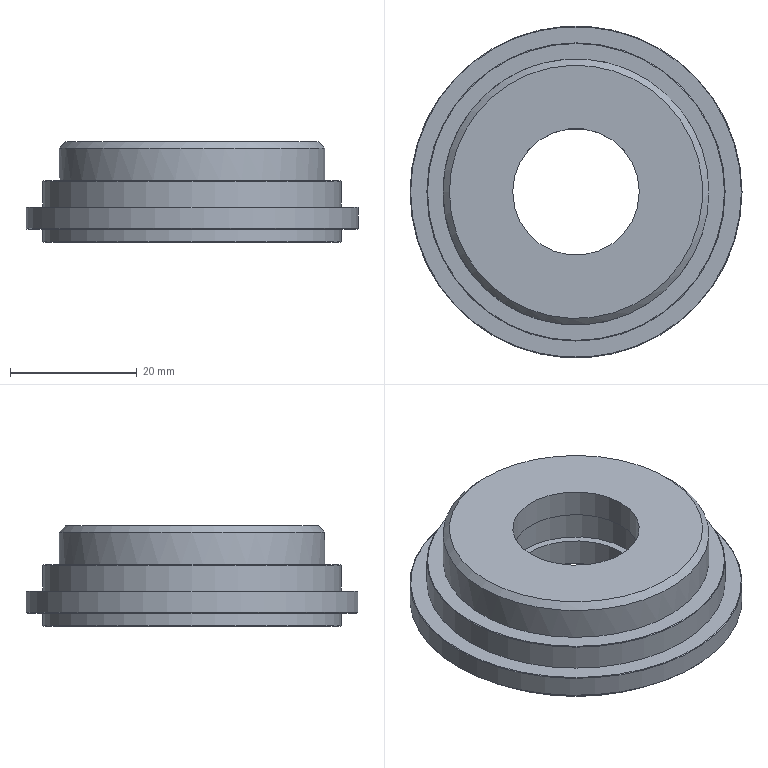Part | NX | features CHAMFER 8, DATUM_CSYS 8, SKETCH 7, EXTRUDE 6, DATUM_PLANE 5, DISTANCE MEASUREMENT 2, Resize Face 2 | 1 solid | 22 faces | box 52.42 x 52.42 x 15.88 mm | volume 19851 mm3 | cylinder 8 | plane 8 | cone 6 | commonest cylinder face diameters 20 x2 47.08 x2 22.22 x1 37.22 x1 41.98 x1 52.42 x1
STEP:
#1=CARTESIAN_POINT('',(10.,0.,11.52));
#2=VERTEX_POINT('',#1);
#3=CARTESIAN_POINT('',(0.,0.,11.52));
#4=DIRECTION('',(0.,0.,1.));
#5=DIRECTION('',(1.,0.,0.));
#6=AXIS2_PLACEMENT_3D('',#3,#4,#5);
#7=CIRCLE('',#6,10.);
#8=EDGE_CURVE('',#2,#2,#7,.T.);
#9=ORIENTED_EDGE('',*,*,#8,.F.);
#10=EDGE_LOOP('',(#9));
#11=FACE_BOUND('',#10,.T.);
#12=CARTESIAN_POINT('',(-10.,0.,15.88));
#13=VERTEX_POINT('',#12);
#14=CARTESIAN_POINT('',(0.,0.,15.88));
#15=DIRECTION('',(0.,0.,-1.));
#16=DIRECTION('',(-1.,0.,0.));
#17=AXIS2_PLACEMENT_3D('',#14,#15,#16);
#18=CIRCLE('',#17,10.);
#19=EDGE_CURVE('',#13,#13,#18,.T.);
#20=ORIENTED_EDGE('',*,*,#19,.F.);
#21=EDGE_LOOP('',(#20));
#22=FACE_BOUND('',#21,.T.);
#23=CARTESIAN_POINT('',(0.,0.,15.88));
#24=DIRECTION('',(0.,0.,-1.));
#25=DIRECTION('',(-1.,0.,0.));
#26=AXIS2_PLACEMENT_3D('',#23,#24,#25);
#27=CYLINDRICAL_SURFACE('',#26,10.);
#28=ADVANCED_FACE('',(#11,#22),#27,.F.);
#29=CARTESIAN_POINT('',(18.61,0.,2.08));
#30=VERTEX_POINT('',#29);
#31=CARTESIAN_POINT('',(0.,0.,2.08));
#32=DIRECTION('',(0.,0.,1.));
#33=DIRECTION('',(1.,0.,0.));
#34=AXIS2_PLACEMENT_3D('',#31,#32,#33);
#35=CIRCLE('',#34,18.61);
#36=EDGE_CURVE('',#30,#30,#35,.F.);
#37=ORIENTED_EDGE('',*,*,#36,.T.);
#38=EDGE_LOOP('',(#37));
#39=FACE_BOUND('',#38,.T.);
#40=CARTESIAN_POINT('',(10.,0.,2.08));
#41=VERTEX_POINT('',#40);
#42=CARTESIAN_POINT('',(0.,0.,2.08));
#43=DIRECTION('',(0.,0.,1.));
#44=DIRECTION('',(1.,0.,0.));
#45=AXIS2_PLACEMENT_3D('',#42,#43,#44);
#46=CIRCLE('',#45,10.);
#47=EDGE_CURVE('',#41,#41,#46,.F.);
#48=ORIENTED_EDGE('',*,*,#47,.F.);
#49=EDGE_LOOP('',(#48));
#50=FACE_BOUND('',#49,.T.);
#51=CARTESIAN_POINT('',(0.,0.,2.08));
#52=DIRECTION('',(0.,0.,1.));
#53=DIRECTION('',(1.,0.,0.));
#54=AXIS2_PLACEMENT_3D('',#51,#52,#53);
#55=PLANE('',#54);
#56=ADVANCED_FACE('',(#39,#50),#55,.F.);
#57=CARTESIAN_POINT('',(26.21,0.,2.18));
#58=VERTEX_POINT('',#57);
#59=CARTESIAN_POINT('',(0.,0.,2.18));
#60=DIRECTION('',(0.,0.,1.));
#61=DIRECTION('',(1.,0.,0.));
#62=AXIS2_PLACEMENT_3D('',#59,#60,#61);
#63=CIRCLE('',#62,26.21);
#64=EDGE_CURVE('',#58,#58,#63,.T.);
#65=ORIENTED_EDGE('',*,*,#64,.T.);
#66=EDGE_LOOP('',(#65));
#67=FACE_BOUND('',#66,.T.);
#68=CARTESIAN_POINT('',(26.21,0.,5.46));
#69=VERTEX_POINT('',#68);
#70=CARTESIAN_POINT('',(0.,0.,5.46));
#71=DIRECTION('',(0.,0.,1.));
#72=DIRECTION('',(1.,0.,0.));
#73=AXIS2_PLACEMENT_3D('',#70,#71,#72);
#74=CIRCLE('',#73,26.21);
#75=EDGE_CURVE('',#69,#69,#74,.F.);
#76=ORIENTED_EDGE('',*,*,#75,.T.);
#77=EDGE_LOOP('',(#76));
#78=FACE_BOUND('',#77,.T.);
#79=CARTESIAN_POINT('',(0.,0.,15.88));
#80=DIRECTION('',(0.,0.,-1.));
#81=DIRECTION('',(-1.,0.,0.));
#82=AXIS2_PLACEMENT_3D('',#79,#80,#81);
#83=CYLINDRICAL_SURFACE('',#82,26.21);
#84=ADVANCED_FACE('',(#67,#78),#83,.T.);
#85=CARTESIAN_POINT('',(-18.71,0.,0.));
#86=VERTEX_POINT('',#85);
#87=CARTESIAN_POINT('',(0.,0.,0.));
#88=DIRECTION('',(0.,0.,-1.));
#89=DIRECTION('',(-1.,0.,0.));
#90=AXIS2_PLACEMENT_3D('',#87,#88,#89);
#91=CIRCLE('',#90,18.71);
#92=EDGE_CURVE('',#86,#86,#91,.F.);
#93=ORIENTED_EDGE('',*,*,#92,.T.);
#94=EDGE_LOOP('',(#93));
#95=FACE_BOUND('',#94,.T.);
#96=CARTESIAN_POINT('',(-23.44,0.,0.));
#97=VERTEX_POINT('',#96);
#98=CARTESIAN_POINT('',(0.,0.,0.));
#99=DIRECTION('',(0.,0.,-1.));
#100=DIRECTION('',(-1.,0.,0.));
#101=AXIS2_PLACEMENT_3D('',#98,#99,#100);
#102=CIRCLE('',#101,23.44);
#103=EDGE_CURVE('',#97,#97,#102,.T.);
#104=ORIENTED_EDGE('',*,*,#103,.T.);
#105=EDGE_LOOP('',(#104));
#106=FACE_BOUND('',#105,.T.);
#107=CARTESIAN_POINT('',(0.,0.,0.));
#108=DIRECTION('',(0.,0.,-1.));
#109=DIRECTION('',(-1.,0.,0.));
#110=AXIS2_PLACEMENT_3D('',#107,#108,#109);
#111=PLANE('',#110);
#112=ADVANCED_FACE('',(#95,#106),#111,.T.);
#113=ORIENTED_EDGE('',*,*,#19,.T.);
#114=EDGE_LOOP('',(#113));
#115=FACE_BOUND('',#114,.T.);
#116=CARTESIAN_POINT('',(-19.99,0.,15.88));
#117=VERTEX_POINT('',#116);
#118=CARTESIAN_POINT('',(0.,0.,15.88));
#119=DIRECTION('',(0.,0.,-1.));
#120=DIRECTION('',(-1.,0.,0.));
#121=AXIS2_PLACEMENT_3D('',#118,#119,#120);
#122=CIRCLE('',#121,19.99);
#123=EDGE_CURVE('',#117,#117,#122,.F.);
#124=ORIENTED_EDGE('',*,*,#123,.T.);
#125=EDGE_LOOP('',(#124));
#126=FACE_BOUND('',#125,.T.);
#127=CARTESIAN_POINT('',(0.,0.,15.88));
#128=DIRECTION('',(0.,0.,-1.));
#129=DIRECTION('',(-1.,0.,0.));
#130=AXIS2_PLACEMENT_3D('',#127,#128,#129);
#131=PLANE('',#130);
#132=ADVANCED_FACE('',(#115,#126),#131,.F.);
#133=ORIENTED_EDGE('',*,*,#47,.T.);
#134=EDGE_LOOP('',(#133));
#135=FACE_BOUND('',#134,.T.);
#136=CARTESIAN_POINT('',(10.,0.,6.44));
#137=VERTEX_POINT('',#136);
#138=CARTESIAN_POINT('',(0.,0.,6.44));
#139=DIRECTION('',(0.,0.,1.));
#140=DIRECTION('',(1.,0.,0.));
#141=AXIS2_PLACEMENT_3D('',#138,#139,#140);
#142=CIRCLE('',#141,10.);
#143=EDGE_CURVE('',#137,#137,#142,.T.);
#144=ORIENTED_EDGE('',*,*,#143,.T.);
#145=EDGE_LOOP('',(#144));
#146=FACE_BOUND('',#145,.T.);
#147=CARTESIAN_POINT('',(0.,0.,15.88));
#148=DIRECTION('',(0.,0.,-1.));
#149=DIRECTION('',(-1.,0.,0.));
#150=AXIS2_PLACEMENT_3D('',#147,#148,#149);
#151=CYLINDRICAL_SURFACE('',#150,10.);
#152=ADVANCED_FACE('',(#135,#146),#151,.F.);
#153=CARTESIAN_POINT('',(11.11,0.,6.44));
#154=VERTEX_POINT('',#153);
#155=CARTESIAN_POINT('',(0.,0.,6.44));
#156=DIRECTION('',(0.,0.,1.));
#157=DIRECTION('',(1.,0.,0.));
#158=AXIS2_PLACEMENT_3D('',#155,#156,#157);
#159=CIRCLE('',#158,11.11);
#160=EDGE_CURVE('',#154,#154,#159,.F.);
#161=ORIENTED_EDGE('',*,*,#160,.T.);
#162=EDGE_LOOP('',(#161));
#163=FACE_BOUND('',#162,.T.);
#164=CARTESIAN_POINT('',(11.11,0.,11.52));
#165=VERTEX_POINT('',#164);
#166=CARTESIAN_POINT('',(0.,0.,11.52));
#167=DIRECTION('',(0.,0.,1.));
#168=DIRECTION('',(1.,0.,0.));
#169=AXIS2_PLACEMENT_3D('',#166,#167,#168);
#170=CIRCLE('',#169,11.11);
#171=EDGE_CURVE('',#165,#165,#170,.F.);
#172=ORIENTED_EDGE('',*,*,#171,.F.);
#173=EDGE_LOOP('',(#172));
#174=FACE_BOUND('',#173,.T.);
#175=CARTESIAN_POINT('',(0.,0.,6.44));
#176=DIRECTION('',(0.,0.,1.));
#177=DIRECTION('',(1.,0.,0.));
#178=AXIS2_PLACEMENT_3D('',#175,#176,#177);
#179=CYLINDRICAL_SURFACE('',#178,11.11);
#180=ADVANCED_FACE('',(#163,#174),#179,.F.);
#181=ORIENTED_EDGE('',*,*,#160,.F.);
#182=EDGE_LOOP('',(#181));
#183=FACE_BOUND('',#182,.T.);
#184=ORIENTED_EDGE('',*,*,#143,.F.);
#185=EDGE_LOOP('',(#184));
#186=FACE_BOUND('',#185,.T.);
#187=CARTESIAN_POINT('',(0.,0.,6.44));
#188=DIRECTION('',(0.,0.,1.));
#189=DIRECTION('',(1.,0.,0.));
#190=AXIS2_PLACEMENT_3D('',#187,#188,#189);
#191=PLANE('',#190);
#192=ADVANCED_FACE('',(#183,#186),#191,.T.);
#193=ORIENTED_EDGE('',*,*,#171,.T.);
#194=EDGE_LOOP('',(#193));
#195=FACE_BOUND('',#194,.T.);
#196=ORIENTED_EDGE('',*,*,#8,.T.);
#197=EDGE_LOOP('',(#196));
#198=FACE_BOUND('',#197,.T.);
#199=CARTESIAN_POINT('',(0.,0.,11.52));
#200=DIRECTION('',(0.,0.,1.));
#201=DIRECTION('',(1.,0.,0.));
#202=AXIS2_PLACEMENT_3D('',#199,#200,#201);
#203=PLANE('',#202);
#204=ADVANCED_FACE('',(#195,#198),#203,.F.);
#205=CARTESIAN_POINT('',(23.54,0.,9.6));
#206=VERTEX_POINT('',#205);
#207=CARTESIAN_POINT('',(0.,0.,9.6));
#208=DIRECTION('',(0.,0.,1.));
#209=DIRECTION('',(1.,0.,0.));
#210=AXIS2_PLACEMENT_3D('',#207,#208,#209);
#211=CIRCLE('',#210,23.54);
#212=EDGE_CURVE('',#206,#206,#211,.F.);
#213=ORIENTED_EDGE('',*,*,#212,.T.);
#214=EDGE_LOOP('',(#213));
#215=FACE_BOUND('',#214,.T.);
#216=CARTESIAN_POINT('',(23.54,0.,5.56));
#217=VERTEX_POINT('',#216);
#218=CARTESIAN_POINT('',(0.,0.,5.56));
#219=DIRECTION('',(0.,0.,1.));
#220=DIRECTION('',(1.,0.,0.));
#221=AXIS2_PLACEMENT_3D('',#218,#219,#220);
#222=CIRCLE('',#221,23.54);
#223=EDGE_CURVE('',#217,#217,#222,.F.);
#224=ORIENTED_EDGE('',*,*,#223,.F.);
#225=EDGE_LOOP('',(#224));
#226=FACE_BOUND('',#225,.T.);
#227=CARTESIAN_POINT('',(0.,0.,5.56));
#228=DIRECTION('',(0.,0.,1.));
#229=DIRECTION('',(1.,0.,0.));
#230=AXIS2_PLACEMENT_3D('',#227,#228,#229);
#231=CYLINDRICAL_SURFACE('',#230,23.54);
#232=ADVANCED_FACE('',(#215,#226),#231,.T.);
#233=CARTESIAN_POINT('',(26.11,0.,5.56));
#234=VERTEX_POINT('',#233);
#235=CARTESIAN_POINT('',(0.,0.,5.56));
#236=DIRECTION('',(0.,0.,1.));
#237=DIRECTION('',(1.,0.,0.));
#238=AXIS2_PLACEMENT_3D('',#235,#236,#237);
#239=CIRCLE('',#238,26.11);
#240=EDGE_CURVE('',#234,#234,#239,.T.);
#241=ORIENTED_EDGE('',*,*,#240,.T.);
#242=EDGE_LOOP('',(#241));
#243=FACE_BOUND('',#242,.T.);
#244=ORIENTED_EDGE('',*,*,#223,.T.);
#245=EDGE_LOOP('',(#244));
#246=FACE_BOUND('',#245,.T.);
#247=CARTESIAN_POINT('',(0.,0.,5.56));
#248=DIRECTION('',(0.,0.,1.));
#249=DIRECTION('',(1.,0.,0.));
#250=AXIS2_PLACEMENT_3D('',#247,#248,#249);
#251=PLANE('',#250);
#252=ADVANCED_FACE('',(#243,#246),#251,.T.);
#253=CARTESIAN_POINT('',(-20.99,0.,14.88));
#254=VERTEX_POINT('',#253);
#255=CARTESIAN_POINT('',(0.,0.,14.88));
#256=DIRECTION('',(0.,0.,-1.));
#257=DIRECTION('',(-1.,0.,0.));
#258=AXIS2_PLACEMENT_3D('',#255,#256,#257);
#259=CIRCLE('',#258,20.99);
#260=EDGE_CURVE('',#254,#254,#259,.T.);
#261=ORIENTED_EDGE('',*,*,#260,.T.);
#262=EDGE_LOOP('',(#261));
#263=FACE_BOUND('',#262,.T.);
#264=CARTESIAN_POINT('',(20.99,0.,9.7));
#265=VERTEX_POINT('',#264);
#266=CARTESIAN_POINT('',(0.,0.,9.7));
#267=DIRECTION('',(0.,0.,1.));
#268=DIRECTION('',(1.,0.,0.));
#269=AXIS2_PLACEMENT_3D('',#266,#267,#268);
#270=CIRCLE('',#269,20.99);
#271=EDGE_CURVE('',#265,#265,#270,.F.);
#272=ORIENTED_EDGE('',*,*,#271,.F.);
#273=EDGE_LOOP('',(#272));
#274=FACE_BOUND('',#273,.T.);
#275=CARTESIAN_POINT('',(0.,0.,9.7));
#276=DIRECTION('',(0.,0.,1.));
#277=DIRECTION('',(1.,0.,0.));
#278=AXIS2_PLACEMENT_3D('',#275,#276,#277);
#279=CYLINDRICAL_SURFACE('',#278,20.99);
#280=ADVANCED_FACE('',(#263,#274),#279,.T.);
#281=CARTESIAN_POINT('',(23.44,0.,9.7));
#282=VERTEX_POINT('',#281);
#283=CARTESIAN_POINT('',(0.,0.,9.7));
#284=DIRECTION('',(0.,0.,1.));
#285=DIRECTION('',(1.,0.,0.));
#286=AXIS2_PLACEMENT_3D('',#283,#284,#285);
#287=CIRCLE('',#286,23.44);
#288=EDGE_CURVE('',#282,#282,#287,.T.);
#289=ORIENTED_EDGE('',*,*,#288,.T.);
#290=EDGE_LOOP('',(#289));
#291=FACE_BOUND('',#290,.T.);
#292=ORIENTED_EDGE('',*,*,#271,.T.);
#293=EDGE_LOOP('',(#292));
#294=FACE_BOUND('',#293,.T.);
#295=CARTESIAN_POINT('',(0.,0.,9.7));
#296=DIRECTION('',(0.,0.,1.));
#297=DIRECTION('',(1.,0.,0.));
#298=AXIS2_PLACEMENT_3D('',#295,#296,#297);
#299=PLANE('',#298);
#300=ADVANCED_FACE('',(#291,#294),#299,.T.);
#301=CARTESIAN_POINT('',(-23.54,0.,0.1));
#302=VERTEX_POINT('',#301);
#303=CARTESIAN_POINT('',(0.,0.,0.1));
#304=DIRECTION('',(0.,0.,-1.));
#305=DIRECTION('',(-1.,0.,0.));
#306=AXIS2_PLACEMENT_3D('',#303,#304,#305);
#307=CIRCLE('',#306,23.54);
#308=EDGE_CURVE('',#302,#302,#307,.F.);
#309=ORIENTED_EDGE('',*,*,#308,.T.);
#310=EDGE_LOOP('',(#309));
#311=FACE_BOUND('',#310,.T.);
#312=CARTESIAN_POINT('',(23.54,0.,2.08));
#313=VERTEX_POINT('',#312);
#314=CARTESIAN_POINT('',(0.,0.,2.08));
#315=DIRECTION('',(0.,0.,1.));
#316=DIRECTION('',(1.,0.,0.));
#317=AXIS2_PLACEMENT_3D('',#314,#315,#316);
#318=CIRCLE('',#317,23.54);
#319=EDGE_CURVE('',#313,#313,#318,.F.);
#320=ORIENTED_EDGE('',*,*,#319,.T.);
#321=EDGE_LOOP('',(#320));
#322=FACE_BOUND('',#321,.T.);
#323=CARTESIAN_POINT('',(0.,0.,2.08));
#324=DIRECTION('',(0.,0.,-1.));
#325=DIRECTION('',(-1.,0.,0.));
#326=AXIS2_PLACEMENT_3D('',#323,#324,#325);
#327=CYLINDRICAL_SURFACE('',#326,23.54);
#328=ADVANCED_FACE('',(#311,#322),#327,.T.);
#329=CARTESIAN_POINT('',(26.11,0.,2.08));
#330=VERTEX_POINT('',#329);
#331=CARTESIAN_POINT('',(0.,0.,2.08));
#332=DIRECTION('',(0.,0.,1.));
#333=DIRECTION('',(1.,0.,0.));
#334=AXIS2_PLACEMENT_3D('',#331,#332,#333);
#335=CIRCLE('',#334,26.11);
#336=EDGE_CURVE('',#330,#330,#335,.F.);
#337=ORIENTED_EDGE('',*,*,#336,.T.);
#338=EDGE_LOOP('',(#337));
#339=FACE_BOUND('',#338,.T.);
#340=ORIENTED_EDGE('',*,*,#319,.F.);
#341=EDGE_LOOP('',(#340));
#342=FACE_BOUND('',#341,.T.);
#343=CARTESIAN_POINT('',(0.,0.,2.08));
#344=DIRECTION('',(0.,0.,1.));
#345=DIRECTION('',(1.,0.,0.));
#346=AXIS2_PLACEMENT_3D('',#343,#344,#345);
#347=PLANE('',#346);
#348=ADVANCED_FACE('',(#339,#342),#347,.F.);
#349=CARTESIAN_POINT('',(-18.61,0.,0.1));
#350=VERTEX_POINT('',#349);
#351=CARTESIAN_POINT('',(0.,0.,0.1));
#352=DIRECTION('',(0.,0.,-1.));
#353=DIRECTION('',(-1.,0.,0.));
#354=AXIS2_PLACEMENT_3D('',#351,#352,#353);
#355=CIRCLE('',#354,18.61);
#356=EDGE_CURVE('',#350,#350,#355,.T.);
#357=ORIENTED_EDGE('',*,*,#356,.T.);
#358=EDGE_LOOP('',(#357));
#359=FACE_BOUND('',#358,.T.);
#360=ORIENTED_EDGE('',*,*,#36,.F.);
#361=EDGE_LOOP('',(#360));
#362=FACE_BOUND('',#361,.T.);
#363=CARTESIAN_POINT('',(0.,0.,2.08));
#364=DIRECTION('',(0.,0.,-1.));
#365=DIRECTION('',(-1.,0.,0.));
#366=AXIS2_PLACEMENT_3D('',#363,#364,#365);
#367=CYLINDRICAL_SURFACE('',#366,18.61);
#368=ADVANCED_FACE('',(#359,#362),#367,.F.);
#369=ORIENTED_EDGE('',*,*,#260,.F.);
#370=EDGE_LOOP('',(#369));
#371=FACE_BOUND('',#370,.T.);
#372=ORIENTED_EDGE('',*,*,#123,.F.);
#373=EDGE_LOOP('',(#372));
#374=FACE_BOUND('',#373,.T.);
#375=CARTESIAN_POINT('',(0.,0.,15.88));
#376=DIRECTION('',(0.,0.,-1.));
#377=DIRECTION('',(-1.,0.,0.));
#378=AXIS2_PLACEMENT_3D('',#375,#376,#377);
#379=CONICAL_SURFACE('',#378,19.99,0.7854);
#380=ADVANCED_FACE('',(#371,#374),#379,.T.);
#381=ORIENTED_EDGE('',*,*,#212,.F.);
#382=EDGE_LOOP('',(#381));
#383=FACE_BOUND('',#382,.T.);
#384=ORIENTED_EDGE('',*,*,#288,.F.);
#385=EDGE_LOOP('',(#384));
#386=FACE_BOUND('',#385,.T.);
#387=CARTESIAN_POINT('',(0.,0.,9.7));
#388=DIRECTION('',(0.,0.,-1.));
#389=DIRECTION('',(-1.,0.,0.));
#390=AXIS2_PLACEMENT_3D('',#387,#388,#389);
#391=CONICAL_SURFACE('',#390,23.44,0.7854);
#392=ADVANCED_FACE('',(#383,#386),#391,.T.);
#393=ORIENTED_EDGE('',*,*,#75,.F.);
#394=EDGE_LOOP('',(#393));
#395=FACE_BOUND('',#394,.T.);
#396=ORIENTED_EDGE('',*,*,#240,.F.);
#397=EDGE_LOOP('',(#396));
#398=FACE_BOUND('',#397,.T.);
#399=CARTESIAN_POINT('',(0.,0.,5.56));
#400=DIRECTION('',(0.,0.,-1.));
#401=DIRECTION('',(-1.,0.,0.));
#402=AXIS2_PLACEMENT_3D('',#399,#400,#401);
#403=CONICAL_SURFACE('',#402,26.11,0.7854);
#404=ADVANCED_FACE('',(#395,#398),#403,.T.);
#405=ORIENTED_EDGE('',*,*,#336,.F.);
#406=EDGE_LOOP('',(#405));
#407=FACE_BOUND('',#406,.T.);
#408=ORIENTED_EDGE('',*,*,#64,.F.);
#409=EDGE_LOOP('',(#408));
#410=FACE_BOUND('',#409,.T.);
#411=CARTESIAN_POINT('',(0.,0.,2.18));
#412=DIRECTION('',(0.,0.,1.));
#413=DIRECTION('',(1.,0.,0.));
#414=AXIS2_PLACEMENT_3D('',#411,#412,#413);
#415=CONICAL_SURFACE('',#414,26.21,0.7854);
#416=ADVANCED_FACE('',(#407,#410),#415,.T.);
#417=ORIENTED_EDGE('',*,*,#103,.F.);
#418=EDGE_LOOP('',(#417));
#419=FACE_BOUND('',#418,.T.);
#420=ORIENTED_EDGE('',*,*,#308,.F.);
#421=EDGE_LOOP('',(#420));
#422=FACE_BOUND('',#421,.T.);
#423=CARTESIAN_POINT('',(0.,0.,0.1));
#424=DIRECTION('',(0.,0.,1.));
#425=DIRECTION('',(1.,0.,0.));
#426=AXIS2_PLACEMENT_3D('',#423,#424,#425);
#427=CONICAL_SURFACE('',#426,23.54,0.7854);
#428=ADVANCED_FACE('',(#419,#422),#427,.T.);
#429=ORIENTED_EDGE('',*,*,#356,.F.);
#430=EDGE_LOOP('',(#429));
#431=FACE_BOUND('',#430,.T.);
#432=ORIENTED_EDGE('',*,*,#92,.F.);
#433=EDGE_LOOP('',(#432));
#434=FACE_BOUND('',#433,.T.);
#435=CARTESIAN_POINT('',(0.,0.,0.));
#436=DIRECTION('',(0.,0.,-1.));
#437=DIRECTION('',(-1.,0.,0.));
#438=AXIS2_PLACEMENT_3D('',#435,#436,#437);
#439=CONICAL_SURFACE('',#438,18.71,0.7854);
#440=ADVANCED_FACE('',(#431,#434),#439,.F.);
#441=CLOSED_SHELL('',(#28,#56,#84,#112,#132,#152,#180,#192,#204,#232,#252,#280,#300,#328,#348,#368,#380,#392,#404,#416,#428,#440));
#442=MANIFOLD_SOLID_BREP('',#441);
#443=(LENGTH_UNIT()NAMED_UNIT(*)SI_UNIT(.MILLI.,.METRE.));
#444=UNCERTAINTY_MEASURE_WITH_UNIT(LENGTH_MEASURE(0.00001),#443,'','');
#445=(NAMED_UNIT(*)PLANE_ANGLE_UNIT()SI_UNIT($,.RADIAN.));
#446=(NAMED_UNIT(*)SI_UNIT($,.STERADIAN.)SOLID_ANGLE_UNIT());
#447=(GEOMETRIC_REPRESENTATION_CONTEXT(3)GLOBAL_UNCERTAINTY_ASSIGNED_CONTEXT((#444))GLOBAL_UNIT_ASSIGNED_CONTEXT((#443,#445,#446))REPRESENTATION_CONTEXT('',''));
#448=ADVANCED_BREP_SHAPE_REPRESENTATION('',(#442),#447);